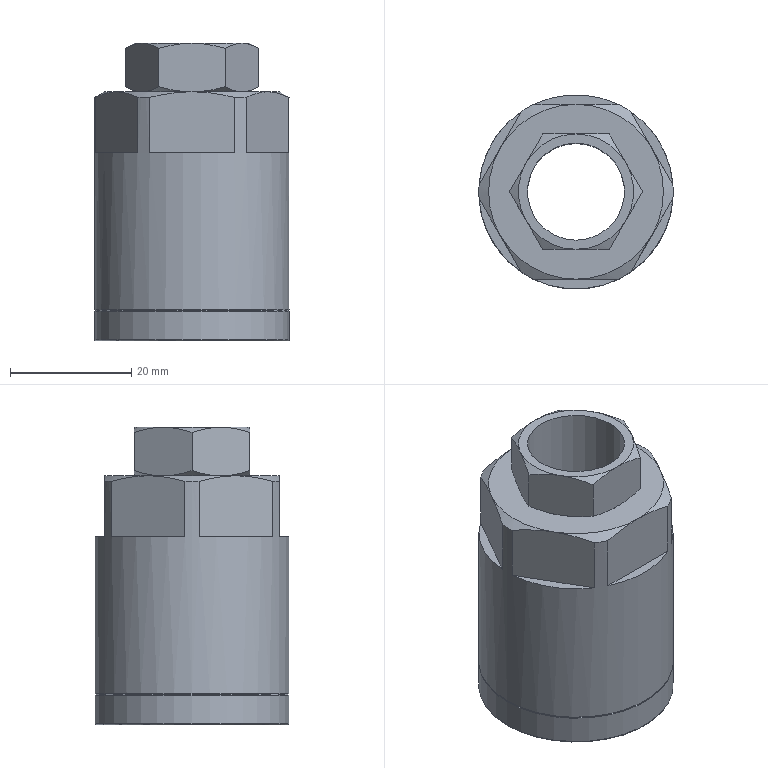Part | STEP file | 冲床-300配套压波_id654_x_t | 1 solid | 45 faces | box 32 x 32 x 49 mm | volume 24682 mm3 | plane 21 | cone 20 | cylinder 3 | torus 1 | commonest cylinder face diameters 32 x2 16 x1
STEP:
#1=CARTESIAN_POINT('',(1821.,0.,307.2));
#2=VERTEX_POINT('',#1);
#3=CARTESIAN_POINT('',(1805.,0.,307.2));
#4=DIRECTION('',(0.,0.,1.));
#5=DIRECTION('',(1.,0.,0.));
#6=AXIS2_PLACEMENT_3D('',#3,#4,#5);
#7=CIRCLE('',#6,16.);
#8=EDGE_CURVE('',#2,#2,#7,.T.);
#9=ORIENTED_EDGE('',*,*,#8,.T.);
#10=EDGE_LOOP('',(#9));
#11=FACE_BOUND('',#10,.T.);
#12=CARTESIAN_POINT('',(1789.,0.,311.9));
#13=VERTEX_POINT('',#12);
#14=CARTESIAN_POINT('',(1805.,0.,311.9));
#15=DIRECTION('',(0.,0.,-1.));
#16=DIRECTION('',(-1.,0.,0.));
#17=AXIS2_PLACEMENT_3D('',#14,#15,#16);
#18=CIRCLE('',#17,16.);
#19=EDGE_CURVE('',#13,#13,#18,.T.);
#20=ORIENTED_EDGE('',*,*,#19,.T.);
#21=EDGE_LOOP('',(#20));
#22=FACE_BOUND('',#21,.T.);
#23=CARTESIAN_POINT('',(1805.,0.,307.));
#24=DIRECTION('',(0.,0.,1.));
#25=DIRECTION('',(-1.,0.,0.));
#26=AXIS2_PLACEMENT_3D('',#23,#24,#25);
#27=CYLINDRICAL_SURFACE('',#26,16.);
#28=ADVANCED_FACE('',(#11,#22),#27,.T.);
#29=CARTESIAN_POINT('',(1813.227,4.75,348.));
#30=VERTEX_POINT('',#29);
#31=CARTESIAN_POINT('',(1805.,9.5,348.));
#32=VERTEX_POINT('',#31);
#33=CARTESIAN_POINT('',(1805.,0.,348.));
#34=DIRECTION('',(0.,0.,1.));
#35=DIRECTION('',(1.,0.,0.));
#36=AXIS2_PLACEMENT_3D('',#33,#34,#35);
#37=CIRCLE('',#36,9.5);
#38=EDGE_CURVE('',#30,#32,#37,.T.);
#39=ORIENTED_EDGE('',*,*,#38,.F.);
#40=CARTESIAN_POINT('',(1813.227,-4.75,348.));
#41=VERTEX_POINT('',#40);
#42=CARTESIAN_POINT('',(1805.,0.,348.));
#43=DIRECTION('',(0.,0.,1.));
#44=DIRECTION('',(1.,0.,0.));
#45=AXIS2_PLACEMENT_3D('',#42,#43,#44);
#46=CIRCLE('',#45,9.5);
#47=EDGE_CURVE('',#41,#30,#46,.T.);
#48=ORIENTED_EDGE('',*,*,#47,.F.);
#49=CARTESIAN_POINT('',(1805.,-9.5,348.));
#50=VERTEX_POINT('',#49);
#51=CARTESIAN_POINT('',(1805.,0.,348.));
#52=DIRECTION('',(0.,0.,1.));
#53=DIRECTION('',(1.,0.,0.));
#54=AXIS2_PLACEMENT_3D('',#51,#52,#53);
#55=CIRCLE('',#54,9.5);
#56=EDGE_CURVE('',#50,#41,#55,.T.);
#57=ORIENTED_EDGE('',*,*,#56,.F.);
#58=CARTESIAN_POINT('',(1796.773,-4.75,348.));
#59=VERTEX_POINT('',#58);
#60=CARTESIAN_POINT('',(1805.,0.,348.));
#61=DIRECTION('',(0.,0.,1.));
#62=DIRECTION('',(1.,0.,0.));
#63=AXIS2_PLACEMENT_3D('',#60,#61,#62);
#64=CIRCLE('',#63,9.5);
#65=EDGE_CURVE('',#59,#50,#64,.T.);
#66=ORIENTED_EDGE('',*,*,#65,.F.);
#67=CARTESIAN_POINT('',(1796.773,4.75,348.));
#68=VERTEX_POINT('',#67);
#69=CARTESIAN_POINT('',(1805.,0.,348.));
#70=DIRECTION('',(0.,0.,1.));
#71=DIRECTION('',(1.,0.,0.));
#72=AXIS2_PLACEMENT_3D('',#69,#70,#71);
#73=CIRCLE('',#72,9.5);
#74=EDGE_CURVE('',#68,#59,#73,.T.);
#75=ORIENTED_EDGE('',*,*,#74,.F.);
#76=CARTESIAN_POINT('',(1805.,0.,348.));
#77=DIRECTION('',(0.,0.,1.));
#78=DIRECTION('',(1.,0.,0.));
#79=AXIS2_PLACEMENT_3D('',#76,#77,#78);
#80=CIRCLE('',#79,9.5);
#81=EDGE_CURVE('',#32,#68,#80,.T.);
#82=ORIENTED_EDGE('',*,*,#81,.F.);
#83=EDGE_LOOP('',(#39,#48,#57,#66,#75,#82));
#84=FACE_BOUND('',#83,.T.);
#85=CARTESIAN_POINT('',(1805.,-14.4,348.));
#86=VERTEX_POINT('',#85);
#87=CARTESIAN_POINT('',(1817.471,-7.2,348.));
#88=VERTEX_POINT('',#87);
#89=CARTESIAN_POINT('',(1805.,0.,348.));
#90=DIRECTION('',(0.,0.,1.));
#91=DIRECTION('',(1.,0.,0.));
#92=AXIS2_PLACEMENT_3D('',#89,#90,#91);
#93=CIRCLE('',#92,14.4);
#94=EDGE_CURVE('',#86,#88,#93,.T.);
#95=ORIENTED_EDGE('',*,*,#94,.T.);
#96=CARTESIAN_POINT('',(1817.471,7.2,348.));
#97=VERTEX_POINT('',#96);
#98=CARTESIAN_POINT('',(1805.,0.,348.));
#99=DIRECTION('',(0.,0.,1.));
#100=DIRECTION('',(1.,0.,0.));
#101=AXIS2_PLACEMENT_3D('',#98,#99,#100);
#102=CIRCLE('',#101,14.4);
#103=EDGE_CURVE('',#88,#97,#102,.T.);
#104=ORIENTED_EDGE('',*,*,#103,.T.);
#105=CARTESIAN_POINT('',(1805.,14.4,348.));
#106=VERTEX_POINT('',#105);
#107=CARTESIAN_POINT('',(1805.,0.,348.));
#108=DIRECTION('',(0.,0.,1.));
#109=DIRECTION('',(1.,0.,0.));
#110=AXIS2_PLACEMENT_3D('',#107,#108,#109);
#111=CIRCLE('',#110,14.4);
#112=EDGE_CURVE('',#97,#106,#111,.T.);
#113=ORIENTED_EDGE('',*,*,#112,.T.);
#114=CARTESIAN_POINT('',(1792.529,7.2,348.));
#115=VERTEX_POINT('',#114);
#116=CARTESIAN_POINT('',(1805.,0.,348.));
#117=DIRECTION('',(0.,0.,1.));
#118=DIRECTION('',(1.,0.,0.));
#119=AXIS2_PLACEMENT_3D('',#116,#117,#118);
#120=CIRCLE('',#119,14.4);
#121=EDGE_CURVE('',#106,#115,#120,.T.);
#122=ORIENTED_EDGE('',*,*,#121,.T.);
#123=CARTESIAN_POINT('',(1792.529,-7.2,348.));
#124=VERTEX_POINT('',#123);
#125=CARTESIAN_POINT('',(1805.,0.,348.));
#126=DIRECTION('',(0.,0.,1.));
#127=DIRECTION('',(1.,0.,0.));
#128=AXIS2_PLACEMENT_3D('',#125,#126,#127);
#129=CIRCLE('',#128,14.4);
#130=EDGE_CURVE('',#115,#124,#129,.T.);
#131=ORIENTED_EDGE('',*,*,#130,.T.);
#132=CARTESIAN_POINT('',(1805.,0.,348.));
#133=DIRECTION('',(0.,0.,1.));
#134=DIRECTION('',(1.,0.,0.));
#135=AXIS2_PLACEMENT_3D('',#132,#133,#134);
#136=CIRCLE('',#135,14.4);
#137=EDGE_CURVE('',#124,#86,#136,.T.);
#138=ORIENTED_EDGE('',*,*,#137,.T.);
#139=EDGE_LOOP('',(#95,#104,#113,#122,#131,#138));
#140=FACE_BOUND('',#139,.T.);
#141=CARTESIAN_POINT('',(1805.,0.,348.));
#142=DIRECTION('',(0.,0.,1.));
#143=DIRECTION('',(-1.,0.,0.));
#144=AXIS2_PLACEMENT_3D('',#141,#142,#143);
#145=PLANE('',#144);
#146=ADVANCED_FACE('',(#84,#140),#145,.T.);
#147=CARTESIAN_POINT('',(1796.016,-13.24,338.));
#148=VERTEX_POINT('',#147);
#149=CARTESIAN_POINT('',(1789.042,-1.16,338.));
#150=VERTEX_POINT('',#149);
#151=CARTESIAN_POINT('',(1796.016,-13.24,338.));
#152=DIRECTION('',(-0.5,0.866,0.));
#153=VECTOR('',#152,1.);
#154=LINE('',#151,#153);
#155=EDGE_CURVE('',#148,#150,#154,.T.);
#156=ORIENTED_EDGE('',*,*,#155,.T.);
#157=CARTESIAN_POINT('',(1805.,0.,338.));
#158=DIRECTION('',(0.,0.,-1.));
#159=DIRECTION('',(0.5,-0.866,0.));
#160=AXIS2_PLACEMENT_3D('',#157,#158,#159);
#161=CIRCLE('',#160,16.);
#162=EDGE_CURVE('',#148,#150,#161,.T.);
#163=ORIENTED_EDGE('',*,*,#162,.F.);
#164=EDGE_LOOP('',(#156,#163));
#165=FACE_OUTER_BOUND('',#164,.T.);
#166=CARTESIAN_POINT('',(1792.529,-7.2,338.));
#167=DIRECTION('',(0.,0.,1.));
#168=DIRECTION('',(-0.5,0.866,0.));
#169=AXIS2_PLACEMENT_3D('',#166,#167,#168);
#170=PLANE('',#169);
#171=ADVANCED_FACE('',(#165),#170,.T.);
#172=CARTESIAN_POINT('',(1796.016,-13.24,347.076));
#173=VERTEX_POINT('',#172);
#174=CARTESIAN_POINT('',(1796.016,-13.24,338.));
#175=DIRECTION('',(0.,0.,-1.));
#176=VECTOR('',#175,1.);
#177=LINE('',#174,#176);
#178=EDGE_CURVE('',#173,#148,#177,.T.);
#179=ORIENTED_EDGE('',*,*,#178,.F.);
#180=CARTESIAN_POINT('',(1796.016,-13.24,347.076));
#181=CARTESIAN_POINT('',(1794.872,-11.257,347.652));
#182=CARTESIAN_POINT('',(1793.712,-9.249,348.));
#183=CARTESIAN_POINT('',(1792.529,-7.2,348.));
#184=B_SPLINE_CURVE_WITH_KNOTS('',3,(#180,#181,#182,#183),.UNSPECIFIED.,.F.,.F.,(4,4),(0.,1.),.UNSPECIFIED.);
#185=EDGE_CURVE('',#173,#124,#184,.T.);
#186=ORIENTED_EDGE('',*,*,#185,.T.);
#187=CARTESIAN_POINT('',(1789.042,-1.16,347.076));
#188=VERTEX_POINT('',#187);
#189=CARTESIAN_POINT('',(1792.529,-7.2,348.));
#190=CARTESIAN_POINT('',(1791.346,-5.151,348.));
#191=CARTESIAN_POINT('',(1790.187,-3.143,347.652));
#192=CARTESIAN_POINT('',(1789.042,-1.16,347.076));
#193=B_SPLINE_CURVE_WITH_KNOTS('',3,(#189,#190,#191,#192),.UNSPECIFIED.,.F.,.F.,(4,4),(0.,1.),.UNSPECIFIED.);
#194=EDGE_CURVE('',#124,#188,#193,.T.);
#195=ORIENTED_EDGE('',*,*,#194,.T.);
#196=CARTESIAN_POINT('',(1789.042,-1.16,338.));
#197=DIRECTION('',(0.,0.,1.));
#198=VECTOR('',#197,1.);
#199=LINE('',#196,#198);
#200=EDGE_CURVE('',#150,#188,#199,.T.);
#201=ORIENTED_EDGE('',*,*,#200,.F.);
#202=ORIENTED_EDGE('',*,*,#155,.F.);
#203=EDGE_LOOP('',(#179,#186,#195,#201,#202));
#204=FACE_OUTER_BOUND('',#203,.T.);
#205=CARTESIAN_POINT('',(1796.016,-13.24,338.));
#206=DIRECTION('',(0.866,0.5,0.));
#207=DIRECTION('',(0.5,-0.866,0.));
#208=AXIS2_PLACEMENT_3D('',#205,#206,#207);
#209=PLANE('',#208);
#210=ADVANCED_FACE('',(#204),#209,.F.);
#211=CARTESIAN_POINT('',(1789.042,1.16,338.));
#212=VERTEX_POINT('',#211);
#213=CARTESIAN_POINT('',(1796.016,13.24,338.));
#214=VERTEX_POINT('',#213);
#215=CARTESIAN_POINT('',(1789.042,1.16,338.));
#216=DIRECTION('',(0.5,0.866,0.));
#217=VECTOR('',#216,1.);
#218=LINE('',#215,#217);
#219=EDGE_CURVE('',#212,#214,#218,.T.);
#220=ORIENTED_EDGE('',*,*,#219,.T.);
#221=CARTESIAN_POINT('',(1805.,0.,338.));
#222=DIRECTION('',(0.,0.,-1.));
#223=DIRECTION('',(-0.5,-0.866,0.));
#224=AXIS2_PLACEMENT_3D('',#221,#222,#223);
#225=CIRCLE('',#224,16.);
#226=EDGE_CURVE('',#212,#214,#225,.T.);
#227=ORIENTED_EDGE('',*,*,#226,.F.);
#228=EDGE_LOOP('',(#220,#227));
#229=FACE_OUTER_BOUND('',#228,.T.);
#230=CARTESIAN_POINT('',(1792.529,7.2,338.));
#231=DIRECTION('',(0.,0.,1.));
#232=DIRECTION('',(0.5,0.866,0.));
#233=AXIS2_PLACEMENT_3D('',#230,#231,#232);
#234=PLANE('',#233);
#235=ADVANCED_FACE('',(#229),#234,.T.);
#236=CARTESIAN_POINT('',(1789.042,1.16,347.076));
#237=VERTEX_POINT('',#236);
#238=CARTESIAN_POINT('',(1789.042,1.16,338.));
#239=DIRECTION('',(0.,0.,1.));
#240=VECTOR('',#239,1.);
#241=LINE('',#238,#240);
#242=EDGE_CURVE('',#212,#237,#241,.T.);
#243=ORIENTED_EDGE('',*,*,#242,.T.);
#244=CARTESIAN_POINT('',(1789.042,1.16,347.076));
#245=CARTESIAN_POINT('',(1790.187,3.143,347.652));
#246=CARTESIAN_POINT('',(1791.346,5.151,348.));
#247=CARTESIAN_POINT('',(1792.529,7.2,348.));
#248=B_SPLINE_CURVE_WITH_KNOTS('',3,(#244,#245,#246,#247),.UNSPECIFIED.,.F.,.F.,(4,4),(0.,1.),.UNSPECIFIED.);
#249=EDGE_CURVE('',#237,#115,#248,.T.);
#250=ORIENTED_EDGE('',*,*,#249,.T.);
#251=CARTESIAN_POINT('',(1796.016,13.24,347.076));
#252=VERTEX_POINT('',#251);
#253=CARTESIAN_POINT('',(1792.529,7.2,348.));
#254=CARTESIAN_POINT('',(1793.712,9.249,348.));
#255=CARTESIAN_POINT('',(1794.872,11.257,347.652));
#256=CARTESIAN_POINT('',(1796.016,13.24,347.076));
#257=B_SPLINE_CURVE_WITH_KNOTS('',3,(#253,#254,#255,#256),.UNSPECIFIED.,.F.,.F.,(4,4),(0.,1.),.UNSPECIFIED.);
#258=EDGE_CURVE('',#115,#252,#257,.T.);
#259=ORIENTED_EDGE('',*,*,#258,.T.);
#260=CARTESIAN_POINT('',(1796.016,13.24,338.));
#261=DIRECTION('',(0.,0.,-1.));
#262=VECTOR('',#261,1.);
#263=LINE('',#260,#262);
#264=EDGE_CURVE('',#252,#214,#263,.T.);
#265=ORIENTED_EDGE('',*,*,#264,.T.);
#266=ORIENTED_EDGE('',*,*,#219,.F.);
#267=EDGE_LOOP('',(#243,#250,#259,#265,#266));
#268=FACE_OUTER_BOUND('',#267,.T.);
#269=CARTESIAN_POINT('',(1789.042,1.16,338.));
#270=DIRECTION('',(0.866,-0.5,0.));
#271=DIRECTION('',(-0.5,-0.866,0.));
#272=AXIS2_PLACEMENT_3D('',#269,#270,#271);
#273=PLANE('',#272);
#274=ADVANCED_FACE('',(#268),#273,.F.);
#275=CARTESIAN_POINT('',(1798.026,14.4,338.));
#276=VERTEX_POINT('',#275);
#277=CARTESIAN_POINT('',(1811.974,14.4,338.));
#278=VERTEX_POINT('',#277);
#279=CARTESIAN_POINT('',(1798.026,14.4,338.));
#280=DIRECTION('',(1.,0.,0.));
#281=VECTOR('',#280,1.);
#282=LINE('',#279,#281);
#283=EDGE_CURVE('',#276,#278,#282,.T.);
#284=ORIENTED_EDGE('',*,*,#283,.T.);
#285=CARTESIAN_POINT('',(1805.,0.,338.));
#286=DIRECTION('',(0.,0.,-1.));
#287=DIRECTION('',(-1.,0.,0.));
#288=AXIS2_PLACEMENT_3D('',#285,#286,#287);
#289=CIRCLE('',#288,16.);
#290=EDGE_CURVE('',#276,#278,#289,.T.);
#291=ORIENTED_EDGE('',*,*,#290,.F.);
#292=EDGE_LOOP('',(#284,#291));
#293=FACE_OUTER_BOUND('',#292,.T.);
#294=CARTESIAN_POINT('',(1805.,14.4,338.));
#295=DIRECTION('',(0.,0.,1.));
#296=DIRECTION('',(1.,0.,0.));
#297=AXIS2_PLACEMENT_3D('',#294,#295,#296);
#298=PLANE('',#297);
#299=ADVANCED_FACE('',(#293),#298,.T.);
#300=CARTESIAN_POINT('',(1798.026,14.4,347.076));
#301=VERTEX_POINT('',#300);
#302=CARTESIAN_POINT('',(1798.026,14.4,338.));
#303=DIRECTION('',(0.,0.,1.));
#304=VECTOR('',#303,1.);
#305=LINE('',#302,#304);
#306=EDGE_CURVE('',#276,#301,#305,.T.);
#307=ORIENTED_EDGE('',*,*,#306,.T.);
#308=CARTESIAN_POINT('',(1798.026,14.4,347.076));
#309=CARTESIAN_POINT('',(1800.315,14.4,347.652));
#310=CARTESIAN_POINT('',(1802.634,14.4,348.));
#311=CARTESIAN_POINT('',(1805.,14.4,348.));
#312=B_SPLINE_CURVE_WITH_KNOTS('',3,(#308,#309,#310,#311),.UNSPECIFIED.,.F.,.F.,(4,4),(0.,1.),.UNSPECIFIED.);
#313=EDGE_CURVE('',#301,#106,#312,.T.);
#314=ORIENTED_EDGE('',*,*,#313,.T.);
#315=CARTESIAN_POINT('',(1811.974,14.4,347.076));
#316=VERTEX_POINT('',#315);
#317=CARTESIAN_POINT('',(1805.,14.4,348.));
#318=CARTESIAN_POINT('',(1807.366,14.4,348.));
#319=CARTESIAN_POINT('',(1809.685,14.4,347.652));
#320=CARTESIAN_POINT('',(1811.974,14.4,347.076));
#321=B_SPLINE_CURVE_WITH_KNOTS('',3,(#317,#318,#319,#320),.UNSPECIFIED.,.F.,.F.,(4,4),(0.,1.),.UNSPECIFIED.);
#322=EDGE_CURVE('',#106,#316,#321,.T.);
#323=ORIENTED_EDGE('',*,*,#322,.T.);
#324=CARTESIAN_POINT('',(1811.974,14.4,338.));
#325=DIRECTION('',(0.,0.,-1.));
#326=VECTOR('',#325,1.);
#327=LINE('',#324,#326);
#328=EDGE_CURVE('',#316,#278,#327,.T.);
#329=ORIENTED_EDGE('',*,*,#328,.T.);
#330=ORIENTED_EDGE('',*,*,#283,.F.);
#331=EDGE_LOOP('',(#307,#314,#323,#329,#330));
#332=FACE_OUTER_BOUND('',#331,.T.);
#333=CARTESIAN_POINT('',(1798.026,14.4,338.));
#334=DIRECTION('',(0.,-1.,0.));
#335=DIRECTION('',(-1.,0.,0.));
#336=AXIS2_PLACEMENT_3D('',#333,#334,#335);
#337=PLANE('',#336);
#338=ADVANCED_FACE('',(#332),#337,.F.);
#339=CARTESIAN_POINT('',(1813.984,13.24,338.));
#340=VERTEX_POINT('',#339);
#341=CARTESIAN_POINT('',(1820.958,1.16,338.));
#342=VERTEX_POINT('',#341);
#343=CARTESIAN_POINT('',(1813.984,13.24,338.));
#344=DIRECTION('',(0.5,-0.866,0.));
#345=VECTOR('',#344,1.);
#346=LINE('',#343,#345);
#347=EDGE_CURVE('',#340,#342,#346,.T.);
#348=ORIENTED_EDGE('',*,*,#347,.T.);
#349=CARTESIAN_POINT('',(1805.,0.,338.));
#350=DIRECTION('',(0.,0.,-1.));
#351=DIRECTION('',(-0.5,0.866,0.));
#352=AXIS2_PLACEMENT_3D('',#349,#350,#351);
#353=CIRCLE('',#352,16.);
#354=EDGE_CURVE('',#340,#342,#353,.T.);
#355=ORIENTED_EDGE('',*,*,#354,.F.);
#356=EDGE_LOOP('',(#348,#355));
#357=FACE_OUTER_BOUND('',#356,.T.);
#358=CARTESIAN_POINT('',(1817.471,7.2,338.));
#359=DIRECTION('',(0.,0.,1.));
#360=DIRECTION('',(0.5,-0.866,0.));
#361=AXIS2_PLACEMENT_3D('',#358,#359,#360);
#362=PLANE('',#361);
#363=ADVANCED_FACE('',(#357),#362,.T.);
#364=CARTESIAN_POINT('',(1813.984,13.24,347.076));
#365=VERTEX_POINT('',#364);
#366=CARTESIAN_POINT('',(1813.984,13.24,338.));
#367=DIRECTION('',(0.,0.,1.));
#368=VECTOR('',#367,1.);
#369=LINE('',#366,#368);
#370=EDGE_CURVE('',#340,#365,#369,.T.);
#371=ORIENTED_EDGE('',*,*,#370,.T.);
#372=CARTESIAN_POINT('',(1813.984,13.24,347.076));
#373=CARTESIAN_POINT('',(1815.128,11.257,347.652));
#374=CARTESIAN_POINT('',(1816.288,9.249,348.));
#375=CARTESIAN_POINT('',(1817.471,7.2,348.));
#376=B_SPLINE_CURVE_WITH_KNOTS('',3,(#372,#373,#374,#375),.UNSPECIFIED.,.F.,.F.,(4,4),(0.,1.),.UNSPECIFIED.);
#377=EDGE_CURVE('',#365,#97,#376,.T.);
#378=ORIENTED_EDGE('',*,*,#377,.T.);
#379=CARTESIAN_POINT('',(1820.958,1.16,347.076));
#380=VERTEX_POINT('',#379);
#381=CARTESIAN_POINT('',(1817.471,7.2,348.));
#382=CARTESIAN_POINT('',(1818.654,5.151,348.));
#383=CARTESIAN_POINT('',(1819.813,3.143,347.652));
#384=CARTESIAN_POINT('',(1820.958,1.16,347.076));
#385=B_SPLINE_CURVE_WITH_KNOTS('',3,(#381,#382,#383,#384),.UNSPECIFIED.,.F.,.F.,(4,4),(0.,1.),.UNSPECIFIED.);
#386=EDGE_CURVE('',#97,#380,#385,.T.);
#387=ORIENTED_EDGE('',*,*,#386,.T.);
#388=CARTESIAN_POINT('',(1820.958,1.16,338.));
#389=DIRECTION('',(0.,0.,-1.));
#390=VECTOR('',#389,1.);
#391=LINE('',#388,#390);
#392=EDGE_CURVE('',#380,#342,#391,.T.);
#393=ORIENTED_EDGE('',*,*,#392,.T.);
#394=ORIENTED_EDGE('',*,*,#347,.F.);
#395=EDGE_LOOP('',(#371,#378,#387,#393,#394));
#396=FACE_OUTER_BOUND('',#395,.T.);
#397=CARTESIAN_POINT('',(1813.984,13.24,338.));
#398=DIRECTION('',(-0.866,-0.5,0.));
#399=DIRECTION('',(-0.5,0.866,0.));
#400=AXIS2_PLACEMENT_3D('',#397,#398,#399);
#401=PLANE('',#400);
#402=ADVANCED_FACE('',(#396),#401,.F.);
#403=CARTESIAN_POINT('',(1820.958,-1.16,338.));
#404=VERTEX_POINT('',#403);
#405=CARTESIAN_POINT('',(1813.984,-13.24,338.));
#406=VERTEX_POINT('',#405);
#407=CARTESIAN_POINT('',(1820.958,-1.16,338.));
#408=DIRECTION('',(-0.5,-0.866,0.));
#409=VECTOR('',#408,1.);
#410=LINE('',#407,#409);
#411=EDGE_CURVE('',#404,#406,#410,.T.);
#412=ORIENTED_EDGE('',*,*,#411,.T.);
#413=CARTESIAN_POINT('',(1805.,0.,338.));
#414=DIRECTION('',(0.,0.,-1.));
#415=DIRECTION('',(0.5,0.866,0.));
#416=AXIS2_PLACEMENT_3D('',#413,#414,#415);
#417=CIRCLE('',#416,16.);
#418=EDGE_CURVE('',#404,#406,#417,.T.);
#419=ORIENTED_EDGE('',*,*,#418,.F.);
#420=EDGE_LOOP('',(#412,#419));
#421=FACE_OUTER_BOUND('',#420,.T.);
#422=CARTESIAN_POINT('',(1817.471,-7.2,338.));
#423=DIRECTION('',(0.,0.,1.));
#424=DIRECTION('',(-0.5,-0.866,0.));
#425=AXIS2_PLACEMENT_3D('',#422,#423,#424);
#426=PLANE('',#425);
#427=ADVANCED_FACE('',(#421),#426,.T.);
#428=CARTESIAN_POINT('',(1820.958,-1.16,347.076));
#429=VERTEX_POINT('',#428);
#430=CARTESIAN_POINT('',(1820.958,-1.16,338.));
#431=DIRECTION('',(0.,0.,-1.));
#432=VECTOR('',#431,1.);
#433=LINE('',#430,#432);
#434=EDGE_CURVE('',#429,#404,#433,.T.);
#435=ORIENTED_EDGE('',*,*,#434,.F.);
#436=CARTESIAN_POINT('',(1820.958,-1.16,347.076));
#437=CARTESIAN_POINT('',(1819.813,-3.143,347.652));
#438=CARTESIAN_POINT('',(1818.654,-5.151,348.));
#439=CARTESIAN_POINT('',(1817.471,-7.2,348.));
#440=B_SPLINE_CURVE_WITH_KNOTS('',3,(#436,#437,#438,#439),.UNSPECIFIED.,.F.,.F.,(4,4),(0.,1.),.UNSPECIFIED.);
#441=EDGE_CURVE('',#429,#88,#440,.T.);
#442=ORIENTED_EDGE('',*,*,#441,.T.);
#443=CARTESIAN_POINT('',(1813.984,-13.24,347.076));
#444=VERTEX_POINT('',#443);
#445=CARTESIAN_POINT('',(1817.471,-7.2,348.));
#446=CARTESIAN_POINT('',(1816.288,-9.249,348.));
#447=CARTESIAN_POINT('',(1815.128,-11.257,347.652));
#448=CARTESIAN_POINT('',(1813.984,-13.24,347.076));
#449=B_SPLINE_CURVE_WITH_KNOTS('',3,(#445,#446,#447,#448),.UNSPECIFIED.,.F.,.F.,(4,4),(0.,1.),.UNSPECIFIED.);
#450=EDGE_CURVE('',#88,#444,#449,.T.);
#451=ORIENTED_EDGE('',*,*,#450,.T.);
#452=CARTESIAN_POINT('',(1813.984,-13.24,338.));
#453=DIRECTION('',(0.,0.,1.));
#454=VECTOR('',#453,1.);
#455=LINE('',#452,#454);
#456=EDGE_CURVE('',#406,#444,#455,.T.);
#457=ORIENTED_EDGE('',*,*,#456,.F.);
#458=ORIENTED_EDGE('',*,*,#411,.F.);
#459=EDGE_LOOP('',(#435,#442,#451,#457,#458));
#460=FACE_OUTER_BOUND('',#459,.T.);
#461=CARTESIAN_POINT('',(1820.958,-1.16,338.));
#462=DIRECTION('',(-0.866,0.5,0.));
#463=DIRECTION('',(0.5,0.866,0.));
#464=AXIS2_PLACEMENT_3D('',#461,#462,#463);
#465=PLANE('',#464);
#466=ADVANCED_FACE('',(#460),#465,.F.);
#467=CARTESIAN_POINT('',(1805.,8.,307.));
#468=VERTEX_POINT('',#467);
#469=CARTESIAN_POINT('',(1805.,0.,307.));
#470=DIRECTION('',(0.,0.,1.));
#471=DIRECTION('',(0.,1.,0.));
#472=AXIS2_PLACEMENT_3D('',#469,#470,#471);
#473=CIRCLE('',#472,8.);
#474=EDGE_CURVE('',#468,#468,#473,.T.);
#475=ORIENTED_EDGE('',*,*,#474,.F.);
#476=EDGE_LOOP('',(#475));
#477=FACE_BOUND('',#476,.T.);
#478=CARTESIAN_POINT('',(1805.,-8.,356.));
#479=VERTEX_POINT('',#478);
#480=CARTESIAN_POINT('',(1805.,0.,356.));
#481=DIRECTION('',(0.,0.,1.));
#482=DIRECTION('',(0.,-1.,0.));
#483=AXIS2_PLACEMENT_3D('',#480,#481,#482);
#484=CIRCLE('',#483,8.);
#485=EDGE_CURVE('',#479,#479,#484,.T.);
#486=ORIENTED_EDGE('',*,*,#485,.T.);
#487=EDGE_LOOP('',(#486));
#488=FACE_BOUND('',#487,.T.);
#489=CARTESIAN_POINT('',(1805.,0.,307.));
#490=DIRECTION('',(0.,0.,1.));
#491=DIRECTION('',(-1.,0.,0.));
#492=AXIS2_PLACEMENT_3D('',#489,#490,#491);
#493=CYLINDRICAL_SURFACE('',#492,8.);
#494=ADVANCED_FACE('',(#477,#488),#493,.F.);
#495=CARTESIAN_POINT('',(1789.,0.,312.1));
#496=VERTEX_POINT('',#495);
#497=CARTESIAN_POINT('',(1805.,0.,312.1));
#498=DIRECTION('',(0.,0.,-1.));
#499=DIRECTION('',(-1.,0.,0.));
#500=AXIS2_PLACEMENT_3D('',#497,#498,#499);
#501=CIRCLE('',#500,16.);
#502=EDGE_CURVE('',#496,#496,#501,.T.);
#503=ORIENTED_EDGE('',*,*,#502,.F.);
#504=EDGE_LOOP('',(#503));
#505=FACE_BOUND('',#504,.T.);
#506=CARTESIAN_POINT('',(1798.026,-14.4,347.076));
#507=VERTEX_POINT('',#506);
#508=CARTESIAN_POINT('',(1805.,0.,347.076));
#509=DIRECTION('',(0.,0.,1.));
#510=DIRECTION('',(-1.,0.,0.));
#511=AXIS2_PLACEMENT_3D('',#508,#509,#510);
#512=CIRCLE('',#511,16.);
#513=EDGE_CURVE('',#173,#507,#512,.T.);
#514=ORIENTED_EDGE('',*,*,#513,.F.);
#515=ORIENTED_EDGE('',*,*,#178,.T.);
#516=ORIENTED_EDGE('',*,*,#162,.T.);
#517=ORIENTED_EDGE('',*,*,#200,.T.);
#518=CARTESIAN_POINT('',(1805.,0.,347.076));
#519=DIRECTION('',(0.,0.,1.));
#520=DIRECTION('',(-1.,0.,0.));
#521=AXIS2_PLACEMENT_3D('',#518,#519,#520);
#522=CIRCLE('',#521,16.);
#523=EDGE_CURVE('',#237,#188,#522,.T.);
#524=ORIENTED_EDGE('',*,*,#523,.F.);
#525=ORIENTED_EDGE('',*,*,#242,.F.);
#526=ORIENTED_EDGE('',*,*,#226,.T.);
#527=ORIENTED_EDGE('',*,*,#264,.F.);
#528=CARTESIAN_POINT('',(1805.,0.,347.076));
#529=DIRECTION('',(0.,0.,1.));
#530=DIRECTION('',(-1.,0.,0.));
#531=AXIS2_PLACEMENT_3D('',#528,#529,#530);
#532=CIRCLE('',#531,16.);
#533=EDGE_CURVE('',#301,#252,#532,.T.);
#534=ORIENTED_EDGE('',*,*,#533,.F.);
#535=ORIENTED_EDGE('',*,*,#306,.F.);
#536=ORIENTED_EDGE('',*,*,#290,.T.);
#537=ORIENTED_EDGE('',*,*,#328,.F.);
#538=CARTESIAN_POINT('',(1805.,0.,347.076));
#539=DIRECTION('',(0.,0.,1.));
#540=DIRECTION('',(-1.,0.,0.));
#541=AXIS2_PLACEMENT_3D('',#538,#539,#540);
#542=CIRCLE('',#541,16.);
#543=EDGE_CURVE('',#365,#316,#542,.T.);
#544=ORIENTED_EDGE('',*,*,#543,.F.);
#545=ORIENTED_EDGE('',*,*,#370,.F.);
#546=ORIENTED_EDGE('',*,*,#354,.T.);
#547=ORIENTED_EDGE('',*,*,#392,.F.);
#548=CARTESIAN_POINT('',(1805.,0.,347.076));
#549=DIRECTION('',(0.,0.,1.));
#550=DIRECTION('',(-1.,0.,0.));
#551=AXIS2_PLACEMENT_3D('',#548,#549,#550);
#552=CIRCLE('',#551,16.);
#553=EDGE_CURVE('',#429,#380,#552,.T.);
#554=ORIENTED_EDGE('',*,*,#553,.F.);
#555=ORIENTED_EDGE('',*,*,#434,.T.);
#556=ORIENTED_EDGE('',*,*,#418,.T.);
#557=ORIENTED_EDGE('',*,*,#456,.T.);
#558=CARTESIAN_POINT('',(1811.974,-14.4,347.076));
#559=VERTEX_POINT('',#558);
#560=CARTESIAN_POINT('',(1805.,0.,347.076));
#561=DIRECTION('',(0.,0.,1.));
#562=DIRECTION('',(-1.,0.,0.));
#563=AXIS2_PLACEMENT_3D('',#560,#561,#562);
#564=CIRCLE('',#563,16.);
#565=EDGE_CURVE('',#559,#444,#564,.T.);
#566=ORIENTED_EDGE('',*,*,#565,.F.);
#567=CARTESIAN_POINT('',(1811.974,-14.4,338.));
#568=VERTEX_POINT('',#567);
#569=CARTESIAN_POINT('',(1811.974,-14.4,338.));
#570=DIRECTION('',(0.,0.,-1.));
#571=VECTOR('',#570,1.);
#572=LINE('',#569,#571);
#573=EDGE_CURVE('',#559,#568,#572,.T.);
#574=ORIENTED_EDGE('',*,*,#573,.T.);
#575=CARTESIAN_POINT('',(1798.026,-14.4,338.));
#576=VERTEX_POINT('',#575);
#577=CARTESIAN_POINT('',(1805.,0.,338.));
#578=DIRECTION('',(0.,0.,-1.));
#579=DIRECTION('',(1.,0.,0.));
#580=AXIS2_PLACEMENT_3D('',#577,#578,#579);
#581=CIRCLE('',#580,16.);
#582=EDGE_CURVE('',#568,#576,#581,.T.);
#583=ORIENTED_EDGE('',*,*,#582,.T.);
#584=CARTESIAN_POINT('',(1798.026,-14.4,338.));
#585=DIRECTION('',(0.,0.,1.));
#586=VECTOR('',#585,1.);
#587=LINE('',#584,#586);
#588=EDGE_CURVE('',#576,#507,#587,.T.);
#589=ORIENTED_EDGE('',*,*,#588,.T.);
#590=EDGE_LOOP('',(#514,#515,#516,#517,#524,#525,#526,#527,#534,#535,#536,#537,#544,#545,#546,#547,#554,#555,#556,#557,#566,#574,#583,#589));
#591=FACE_BOUND('',#590,.T.);
#592=CARTESIAN_POINT('',(1805.,0.,307.));
#593=DIRECTION('',(0.,0.,1.));
#594=DIRECTION('',(-1.,0.,0.));
#595=AXIS2_PLACEMENT_3D('',#592,#593,#594);
#596=CYLINDRICAL_SURFACE('',#595,16.);
#597=ADVANCED_FACE('',(#505,#591),#596,.T.);
#598=CARTESIAN_POINT('',(1820.8,0.,307.));
#599=VERTEX_POINT('',#598);
#600=CARTESIAN_POINT('',(1805.,0.,307.));
#601=DIRECTION('',(0.,0.,-1.));
#602=DIRECTION('',(1.,0.,0.));
#603=AXIS2_PLACEMENT_3D('',#600,#601,#602);
#604=CIRCLE('',#603,15.8);
#605=EDGE_CURVE('',#599,#599,#604,.T.);
#606=ORIENTED_EDGE('',*,*,#605,.T.);
#607=EDGE_LOOP('',(#606));
#608=FACE_BOUND('',#607,.T.);
#609=ORIENTED_EDGE('',*,*,#474,.T.);
#610=EDGE_LOOP('',(#609));
#611=FACE_BOUND('',#610,.T.);
#612=CARTESIAN_POINT('',(1805.,0.,307.));
#613=DIRECTION('',(0.,0.,1.));
#614=DIRECTION('',(-1.,0.,0.));
#615=AXIS2_PLACEMENT_3D('',#612,#613,#614);
#616=PLANE('',#615);
#617=ADVANCED_FACE('',(#608,#611),#616,.F.);
#618=CARTESIAN_POINT('',(1811.974,-14.4,338.));
#619=DIRECTION('',(-1.,0.,0.));
#620=VECTOR('',#619,1.);
#621=LINE('',#618,#620);
#622=EDGE_CURVE('',#568,#576,#621,.T.);
#623=ORIENTED_EDGE('',*,*,#622,.T.);
#624=ORIENTED_EDGE('',*,*,#582,.F.);
#625=EDGE_LOOP('',(#623,#624));
#626=FACE_OUTER_BOUND('',#625,.T.);
#627=CARTESIAN_POINT('',(1805.,-14.4,338.));
#628=DIRECTION('',(0.,0.,1.));
#629=DIRECTION('',(-1.,0.,0.));
#630=AXIS2_PLACEMENT_3D('',#627,#628,#629);
#631=PLANE('',#630);
#632=ADVANCED_FACE('',(#626),#631,.T.);
#633=ORIENTED_EDGE('',*,*,#573,.F.);
#634=CARTESIAN_POINT('',(1811.974,-14.4,347.076));
#635=CARTESIAN_POINT('',(1809.685,-14.4,347.652));
#636=CARTESIAN_POINT('',(1807.366,-14.4,348.));
#637=CARTESIAN_POINT('',(1805.,-14.4,348.));
#638=B_SPLINE_CURVE_WITH_KNOTS('',3,(#634,#635,#636,#637),.UNSPECIFIED.,.F.,.F.,(4,4),(0.,1.),.UNSPECIFIED.);
#639=EDGE_CURVE('',#559,#86,#638,.T.);
#640=ORIENTED_EDGE('',*,*,#639,.T.);
#641=CARTESIAN_POINT('',(1805.,-14.4,348.));
#642=CARTESIAN_POINT('',(1802.634,-14.4,348.));
#643=CARTESIAN_POINT('',(1800.315,-14.4,347.652));
#644=CARTESIAN_POINT('',(1798.026,-14.4,347.076));
#645=B_SPLINE_CURVE_WITH_KNOTS('',3,(#641,#642,#643,#644),.UNSPECIFIED.,.F.,.F.,(4,4),(0.,1.),.UNSPECIFIED.);
#646=EDGE_CURVE('',#86,#507,#645,.T.);
#647=ORIENTED_EDGE('',*,*,#646,.T.);
#648=ORIENTED_EDGE('',*,*,#588,.F.);
#649=ORIENTED_EDGE('',*,*,#622,.F.);
#650=EDGE_LOOP('',(#633,#640,#647,#648,#649));
#651=FACE_OUTER_BOUND('',#650,.T.);
#652=CARTESIAN_POINT('',(1811.974,-14.4,338.));
#653=DIRECTION('',(0.,1.,0.));
#654=DIRECTION('',(1.,0.,0.));
#655=AXIS2_PLACEMENT_3D('',#652,#653,#654);
#656=PLANE('',#655);
#657=ADVANCED_FACE('',(#651),#656,.F.);
#658=ORIENTED_EDGE('',*,*,#513,.T.);
#659=ORIENTED_EDGE('',*,*,#646,.F.);
#660=ORIENTED_EDGE('',*,*,#137,.F.);
#661=ORIENTED_EDGE('',*,*,#185,.F.);
#662=EDGE_LOOP('',(#658,#659,#660,#661));
#663=FACE_OUTER_BOUND('',#662,.T.);
#664=CARTESIAN_POINT('',(1805.,0.,345.5));
#665=DIRECTION('',(0.,0.,-1.));
#666=DIRECTION('',(1.,0.,0.));
#667=AXIS2_PLACEMENT_3D('',#664,#665,#666);
#668=CONICAL_SURFACE('',#667,18.73,60.);
#669=ADVANCED_FACE('',(#663),#668,.T.);
#670=ORIENTED_EDGE('',*,*,#94,.F.);
#671=ORIENTED_EDGE('',*,*,#639,.F.);
#672=ORIENTED_EDGE('',*,*,#565,.T.);
#673=ORIENTED_EDGE('',*,*,#450,.F.);
#674=EDGE_LOOP('',(#670,#671,#672,#673));
#675=FACE_OUTER_BOUND('',#674,.T.);
#676=CARTESIAN_POINT('',(1805.,0.,345.5));
#677=DIRECTION('',(0.,0.,-1.));
#678=DIRECTION('',(1.,0.,0.));
#679=AXIS2_PLACEMENT_3D('',#676,#677,#678);
#680=CONICAL_SURFACE('',#679,18.73,60.);
#681=ADVANCED_FACE('',(#675),#680,.T.);
#682=ORIENTED_EDGE('',*,*,#103,.F.);
#683=ORIENTED_EDGE('',*,*,#441,.F.);
#684=ORIENTED_EDGE('',*,*,#553,.T.);
#685=ORIENTED_EDGE('',*,*,#386,.F.);
#686=EDGE_LOOP('',(#682,#683,#684,#685));
#687=FACE_OUTER_BOUND('',#686,.T.);
#688=CARTESIAN_POINT('',(1805.,0.,345.5));
#689=DIRECTION('',(0.,0.,-1.));
#690=DIRECTION('',(1.,0.,0.));
#691=AXIS2_PLACEMENT_3D('',#688,#689,#690);
#692=CONICAL_SURFACE('',#691,18.73,60.);
#693=ADVANCED_FACE('',(#687),#692,.T.);
#694=ORIENTED_EDGE('',*,*,#112,.F.);
#695=ORIENTED_EDGE('',*,*,#377,.F.);
#696=ORIENTED_EDGE('',*,*,#543,.T.);
#697=ORIENTED_EDGE('',*,*,#322,.F.);
#698=EDGE_LOOP('',(#694,#695,#696,#697));
#699=FACE_OUTER_BOUND('',#698,.T.);
#700=CARTESIAN_POINT('',(1805.,0.,345.5));
#701=DIRECTION('',(0.,0.,-1.));
#702=DIRECTION('',(1.,0.,0.));
#703=AXIS2_PLACEMENT_3D('',#700,#701,#702);
#704=CONICAL_SURFACE('',#703,18.73,60.);
#705=ADVANCED_FACE('',(#699),#704,.T.);
#706=ORIENTED_EDGE('',*,*,#121,.F.);
#707=ORIENTED_EDGE('',*,*,#313,.F.);
#708=ORIENTED_EDGE('',*,*,#533,.T.);
#709=ORIENTED_EDGE('',*,*,#258,.F.);
#710=EDGE_LOOP('',(#706,#707,#708,#709));
#711=FACE_OUTER_BOUND('',#710,.T.);
#712=CARTESIAN_POINT('',(1805.,0.,345.5));
#713=DIRECTION('',(0.,0.,-1.));
#714=DIRECTION('',(1.,0.,0.));
#715=AXIS2_PLACEMENT_3D('',#712,#713,#714);
#716=CONICAL_SURFACE('',#715,18.73,60.);
#717=ADVANCED_FACE('',(#711),#716,.T.);
#718=ORIENTED_EDGE('',*,*,#523,.T.);
#719=ORIENTED_EDGE('',*,*,#194,.F.);
#720=ORIENTED_EDGE('',*,*,#130,.F.);
#721=ORIENTED_EDGE('',*,*,#249,.F.);
#722=EDGE_LOOP('',(#718,#719,#720,#721));
#723=FACE_OUTER_BOUND('',#722,.T.);
#724=CARTESIAN_POINT('',(1805.,0.,345.5));
#725=DIRECTION('',(0.,0.,-1.));
#726=DIRECTION('',(1.,0.,0.));
#727=AXIS2_PLACEMENT_3D('',#724,#725,#726);
#728=CONICAL_SURFACE('',#727,18.73,60.);
#729=ADVANCED_FACE('',(#723),#728,.T.);
#730=ORIENTED_EDGE('',*,*,#19,.F.);
#731=EDGE_LOOP('',(#730));
#732=FACE_BOUND('',#731,.T.);
#733=CARTESIAN_POINT('',(1789.173,0.,312.));
#734=VERTEX_POINT('',#733);
#735=CARTESIAN_POINT('',(1805.,0.,312.));
#736=DIRECTION('',(0.,0.,-1.));
#737=DIRECTION('',(-1.,0.,0.));
#738=AXIS2_PLACEMENT_3D('',#735,#736,#737);
#739=CIRCLE('',#738,15.827);
#740=EDGE_CURVE('',#734,#734,#739,.T.);
#741=ORIENTED_EDGE('',*,*,#740,.T.);
#742=EDGE_LOOP('',(#741));
#743=FACE_BOUND('',#742,.T.);
#744=CARTESIAN_POINT('',(1805.,0.,312.));
#745=DIRECTION('',(0.,0.,-1.));
#746=DIRECTION('',(1.,0.,0.));
#747=AXIS2_PLACEMENT_3D('',#744,#745,#746);
#748=CONICAL_SURFACE('',#747,15.827,60.);
#749=ADVANCED_FACE('',(#732,#743),#748,.T.);
#750=ORIENTED_EDGE('',*,*,#740,.F.);
#751=EDGE_LOOP('',(#750));
#752=FACE_BOUND('',#751,.T.);
#753=ORIENTED_EDGE('',*,*,#502,.T.);
#754=EDGE_LOOP('',(#753));
#755=FACE_BOUND('',#754,.T.);
#756=CARTESIAN_POINT('',(1805.,0.,312.1));
#757=DIRECTION('',(0.,0.,1.));
#758=DIRECTION('',(-1.,0.,0.));
#759=AXIS2_PLACEMENT_3D('',#756,#757,#758);
#760=CONICAL_SURFACE('',#759,16.,60.);
#761=ADVANCED_FACE('',(#752,#755),#760,.T.);
#762=ORIENTED_EDGE('',*,*,#605,.F.);
#763=EDGE_LOOP('',(#762));
#764=FACE_BOUND('',#763,.T.);
#765=ORIENTED_EDGE('',*,*,#8,.F.);
#766=EDGE_LOOP('',(#765));
#767=FACE_BOUND('',#766,.T.);
#768=CARTESIAN_POINT('',(1805.,0.,307.2));
#769=DIRECTION('',(0.,0.,1.));
#770=DIRECTION('',(-1.,0.,0.));
#771=AXIS2_PLACEMENT_3D('',#768,#769,#770);
#772=TOROIDAL_SURFACE('',#771,15.8,0.2);
#773=ADVANCED_FACE('',(#764,#767),#772,.T.);
#774=CARTESIAN_POINT('',(1799.515,-9.5,348.849));
#775=VERTEX_POINT('',#774);
#776=CARTESIAN_POINT('',(1799.515,-9.5,355.151));
#777=VERTEX_POINT('',#776);
#778=CARTESIAN_POINT('',(1799.515,-9.5,348.));
#779=DIRECTION('',(0.,0.,1.));
#780=VECTOR('',#779,1.);
#781=LINE('',#778,#780);
#782=EDGE_CURVE('',#775,#777,#781,.T.);
#783=ORIENTED_EDGE('',*,*,#782,.F.);
#784=CARTESIAN_POINT('',(1799.515,-9.5,348.849));
#785=CARTESIAN_POINT('',(1801.307,-9.5,348.331));
#786=CARTESIAN_POINT('',(1803.128,-9.5,348.));
#787=CARTESIAN_POINT('',(1805.,-9.5,348.));
#788=B_SPLINE_CURVE_WITH_KNOTS('',3,(#784,#785,#786,#787),.UNSPECIFIED.,.F.,.F.,(4,4),(0.,1.),.UNSPECIFIED.);
#789=EDGE_CURVE('',#775,#50,#788,.T.);
#790=ORIENTED_EDGE('',*,*,#789,.T.);
#791=CARTESIAN_POINT('',(1810.485,-9.5,348.849));
#792=VERTEX_POINT('',#791);
#793=CARTESIAN_POINT('',(1805.,-9.5,348.));
#794=CARTESIAN_POINT('',(1806.872,-9.5,348.));
#795=CARTESIAN_POINT('',(1808.693,-9.5,348.331));
#796=CARTESIAN_POINT('',(1810.485,-9.5,348.849));
#797=B_SPLINE_CURVE_WITH_KNOTS('',3,(#793,#794,#795,#796),.UNSPECIFIED.,.F.,.F.,(4,4),(0.,1.),.UNSPECIFIED.);
#798=EDGE_CURVE('',#50,#792,#797,.T.);
#799=ORIENTED_EDGE('',*,*,#798,.T.);
#800=CARTESIAN_POINT('',(1810.485,-9.5,355.151));
#801=VERTEX_POINT('',#800);
#802=CARTESIAN_POINT('',(1810.485,-9.5,348.));
#803=DIRECTION('',(0.,0.,1.));
#804=VECTOR('',#803,1.);
#805=LINE('',#802,#804);
#806=EDGE_CURVE('',#792,#801,#805,.T.);
#807=ORIENTED_EDGE('',*,*,#806,.T.);
#808=CARTESIAN_POINT('',(1805.,-9.5,356.));
#809=VERTEX_POINT('',#808);
#810=CARTESIAN_POINT('',(1805.,-9.5,356.));
#811=CARTESIAN_POINT('',(1806.872,-9.5,356.));
#812=CARTESIAN_POINT('',(1808.693,-9.5,355.669));
#813=CARTESIAN_POINT('',(1810.485,-9.5,355.151));
#814=B_SPLINE_CURVE_WITH_KNOTS('',3,(#810,#811,#812,#813),.UNSPECIFIED.,.F.,.F.,(4,4),(0.,1.),.UNSPECIFIED.);
#815=EDGE_CURVE('',#809,#801,#814,.T.);
#816=ORIENTED_EDGE('',*,*,#815,.F.);
#817=CARTESIAN_POINT('',(1799.515,-9.5,355.151));
#818=CARTESIAN_POINT('',(1801.307,-9.5,355.669));
#819=CARTESIAN_POINT('',(1803.128,-9.5,356.));
#820=CARTESIAN_POINT('',(1805.,-9.5,356.));
#821=B_SPLINE_CURVE_WITH_KNOTS('',3,(#817,#818,#819,#820),.UNSPECIFIED.,.F.,.F.,(4,4),(0.,1.),.UNSPECIFIED.);
#822=EDGE_CURVE('',#777,#809,#821,.T.);
#823=ORIENTED_EDGE('',*,*,#822,.F.);
#824=EDGE_LOOP('',(#783,#790,#799,#807,#816,#823));
#825=FACE_OUTER_BOUND('',#824,.T.);
#826=CARTESIAN_POINT('',(1799.515,-9.5,348.));
#827=DIRECTION('',(0.,-1.,0.));
#828=DIRECTION('',(-1.,0.,0.));
#829=AXIS2_PLACEMENT_3D('',#826,#827,#828);
#830=PLANE('',#829);
#831=ADVANCED_FACE('',(#825),#830,.T.);
#832=ORIENTED_EDGE('',*,*,#806,.F.);
#833=CARTESIAN_POINT('',(1810.485,-9.5,348.849));
#834=CARTESIAN_POINT('',(1811.381,-7.948,348.331));
#835=CARTESIAN_POINT('',(1812.291,-6.371,348.));
#836=CARTESIAN_POINT('',(1813.227,-4.75,348.));
#837=B_SPLINE_CURVE_WITH_KNOTS('',3,(#833,#834,#835,#836),.UNSPECIFIED.,.F.,.F.,(4,4),(0.,1.),.UNSPECIFIED.);
#838=EDGE_CURVE('',#792,#41,#837,.T.);
#839=ORIENTED_EDGE('',*,*,#838,.T.);
#840=CARTESIAN_POINT('',(1815.97,0.,348.849));
#841=VERTEX_POINT('',#840);
#842=CARTESIAN_POINT('',(1813.227,-4.75,348.));
#843=CARTESIAN_POINT('',(1814.163,-3.129,348.));
#844=CARTESIAN_POINT('',(1815.074,-1.552,348.331));
#845=CARTESIAN_POINT('',(1815.97,0.,348.849));
#846=B_SPLINE_CURVE_WITH_KNOTS('',3,(#842,#843,#844,#845),.UNSPECIFIED.,.F.,.F.,(4,4),(0.,1.),.UNSPECIFIED.);
#847=EDGE_CURVE('',#41,#841,#846,.T.);
#848=ORIENTED_EDGE('',*,*,#847,.T.);
#849=CARTESIAN_POINT('',(1815.97,0.,355.151));
#850=VERTEX_POINT('',#849);
#851=CARTESIAN_POINT('',(1815.97,0.,348.));
#852=DIRECTION('',(0.,0.,1.));
#853=VECTOR('',#852,1.);
#854=LINE('',#851,#853);
#855=EDGE_CURVE('',#841,#850,#854,.T.);
#856=ORIENTED_EDGE('',*,*,#855,.T.);
#857=CARTESIAN_POINT('',(1813.227,-4.75,356.));
#858=VERTEX_POINT('',#857);
#859=CARTESIAN_POINT('',(1813.227,-4.75,356.));
#860=CARTESIAN_POINT('',(1814.163,-3.129,356.));
#861=CARTESIAN_POINT('',(1815.074,-1.552,355.669));
#862=CARTESIAN_POINT('',(1815.97,0.,355.151));
#863=B_SPLINE_CURVE_WITH_KNOTS('',3,(#859,#860,#861,#862),.UNSPECIFIED.,.F.,.F.,(4,4),(0.,1.),.UNSPECIFIED.);
#864=EDGE_CURVE('',#858,#850,#863,.T.);
#865=ORIENTED_EDGE('',*,*,#864,.F.);
#866=CARTESIAN_POINT('',(1810.485,-9.5,355.151));
#867=CARTESIAN_POINT('',(1811.381,-7.948,355.669));
#868=CARTESIAN_POINT('',(1812.291,-6.371,356.));
#869=CARTESIAN_POINT('',(1813.227,-4.75,356.));
#870=B_SPLINE_CURVE_WITH_KNOTS('',3,(#866,#867,#868,#869),.UNSPECIFIED.,.F.,.F.,(4,4),(0.,1.),.UNSPECIFIED.);
#871=EDGE_CURVE('',#801,#858,#870,.T.);
#872=ORIENTED_EDGE('',*,*,#871,.F.);
#873=EDGE_LOOP('',(#832,#839,#848,#856,#865,#872));
#874=FACE_OUTER_BOUND('',#873,.T.);
#875=CARTESIAN_POINT('',(1810.485,-9.5,348.));
#876=DIRECTION('',(0.866,-0.5,0.));
#877=DIRECTION('',(-0.5,-0.866,0.));
#878=AXIS2_PLACEMENT_3D('',#875,#876,#877);
#879=PLANE('',#878);
#880=ADVANCED_FACE('',(#874),#879,.T.);
#881=ORIENTED_EDGE('',*,*,#855,.F.);
#882=CARTESIAN_POINT('',(1815.97,0.,348.849));
#883=CARTESIAN_POINT('',(1815.074,1.552,348.331));
#884=CARTESIAN_POINT('',(1814.163,3.129,348.));
#885=CARTESIAN_POINT('',(1813.227,4.75,348.));
#886=B_SPLINE_CURVE_WITH_KNOTS('',3,(#882,#883,#884,#885),.UNSPECIFIED.,.F.,.F.,(4,4),(0.,1.),.UNSPECIFIED.);
#887=EDGE_CURVE('',#841,#30,#886,.T.);
#888=ORIENTED_EDGE('',*,*,#887,.T.);
#889=CARTESIAN_POINT('',(1810.485,9.5,348.849));
#890=VERTEX_POINT('',#889);
#891=CARTESIAN_POINT('',(1813.227,4.75,348.));
#892=CARTESIAN_POINT('',(1812.291,6.371,348.));
#893=CARTESIAN_POINT('',(1811.381,7.948,348.331));
#894=CARTESIAN_POINT('',(1810.485,9.5,348.849));
#895=B_SPLINE_CURVE_WITH_KNOTS('',3,(#891,#892,#893,#894),.UNSPECIFIED.,.F.,.F.,(4,4),(0.,1.),.UNSPECIFIED.);
#896=EDGE_CURVE('',#30,#890,#895,.T.);
#897=ORIENTED_EDGE('',*,*,#896,.T.);
#898=CARTESIAN_POINT('',(1810.485,9.5,355.151));
#899=VERTEX_POINT('',#898);
#900=CARTESIAN_POINT('',(1810.485,9.5,348.));
#901=DIRECTION('',(0.,0.,1.));
#902=VECTOR('',#901,1.);
#903=LINE('',#900,#902);
#904=EDGE_CURVE('',#890,#899,#903,.T.);
#905=ORIENTED_EDGE('',*,*,#904,.T.);
#906=CARTESIAN_POINT('',(1813.227,4.75,356.));
#907=VERTEX_POINT('',#906);
#908=CARTESIAN_POINT('',(1813.227,4.75,356.));
#909=CARTESIAN_POINT('',(1812.291,6.371,356.));
#910=CARTESIAN_POINT('',(1811.381,7.948,355.669));
#911=CARTESIAN_POINT('',(1810.485,9.5,355.151));
#912=B_SPLINE_CURVE_WITH_KNOTS('',3,(#908,#909,#910,#911),.UNSPECIFIED.,.F.,.F.,(4,4),(0.,1.),.UNSPECIFIED.);
#913=EDGE_CURVE('',#907,#899,#912,.T.);
#914=ORIENTED_EDGE('',*,*,#913,.F.);
#915=CARTESIAN_POINT('',(1815.97,0.,355.151));
#916=CARTESIAN_POINT('',(1815.074,1.552,355.669));
#917=CARTESIAN_POINT('',(1814.163,3.129,356.));
#918=CARTESIAN_POINT('',(1813.227,4.75,356.));
#919=B_SPLINE_CURVE_WITH_KNOTS('',3,(#915,#916,#917,#918),.UNSPECIFIED.,.F.,.F.,(4,4),(0.,1.),.UNSPECIFIED.);
#920=EDGE_CURVE('',#850,#907,#919,.T.);
#921=ORIENTED_EDGE('',*,*,#920,.F.);
#922=EDGE_LOOP('',(#881,#888,#897,#905,#914,#921));
#923=FACE_OUTER_BOUND('',#922,.T.);
#924=CARTESIAN_POINT('',(1815.97,0.,348.));
#925=DIRECTION('',(0.866,0.5,0.));
#926=DIRECTION('',(0.5,-0.866,0.));
#927=AXIS2_PLACEMENT_3D('',#924,#925,#926);
#928=PLANE('',#927);
#929=ADVANCED_FACE('',(#923),#928,.T.);
#930=ORIENTED_EDGE('',*,*,#904,.F.);
#931=CARTESIAN_POINT('',(1810.485,9.5,348.849));
#932=CARTESIAN_POINT('',(1808.693,9.5,348.331));
#933=CARTESIAN_POINT('',(1806.872,9.5,348.));
#934=CARTESIAN_POINT('',(1805.,9.5,348.));
#935=B_SPLINE_CURVE_WITH_KNOTS('',3,(#931,#932,#933,#934),.UNSPECIFIED.,.F.,.F.,(4,4),(0.,1.),.UNSPECIFIED.);
#936=EDGE_CURVE('',#890,#32,#935,.T.);
#937=ORIENTED_EDGE('',*,*,#936,.T.);
#938=CARTESIAN_POINT('',(1799.515,9.5,348.849));
#939=VERTEX_POINT('',#938);
#940=CARTESIAN_POINT('',(1805.,9.5,348.));
#941=CARTESIAN_POINT('',(1803.128,9.5,348.));
#942=CARTESIAN_POINT('',(1801.307,9.5,348.331));
#943=CARTESIAN_POINT('',(1799.515,9.5,348.849));
#944=B_SPLINE_CURVE_WITH_KNOTS('',3,(#940,#941,#942,#943),.UNSPECIFIED.,.F.,.F.,(4,4),(0.,1.),.UNSPECIFIED.);
#945=EDGE_CURVE('',#32,#939,#944,.T.);
#946=ORIENTED_EDGE('',*,*,#945,.T.);
#947=CARTESIAN_POINT('',(1799.515,9.5,355.151));
#948=VERTEX_POINT('',#947);
#949=CARTESIAN_POINT('',(1799.515,9.5,348.));
#950=DIRECTION('',(0.,0.,1.));
#951=VECTOR('',#950,1.);
#952=LINE('',#949,#951);
#953=EDGE_CURVE('',#939,#948,#952,.T.);
#954=ORIENTED_EDGE('',*,*,#953,.T.);
#955=CARTESIAN_POINT('',(1805.,9.5,356.));
#956=VERTEX_POINT('',#955);
#957=CARTESIAN_POINT('',(1805.,9.5,356.));
#958=CARTESIAN_POINT('',(1803.128,9.5,356.));
#959=CARTESIAN_POINT('',(1801.307,9.5,355.669));
#960=CARTESIAN_POINT('',(1799.515,9.5,355.151));
#961=B_SPLINE_CURVE_WITH_KNOTS('',3,(#957,#958,#959,#960),.UNSPECIFIED.,.F.,.F.,(4,4),(0.,1.),.UNSPECIFIED.);
#962=EDGE_CURVE('',#956,#948,#961,.T.);
#963=ORIENTED_EDGE('',*,*,#962,.F.);
#964=CARTESIAN_POINT('',(1810.485,9.5,355.151));
#965=CARTESIAN_POINT('',(1808.693,9.5,355.669));
#966=CARTESIAN_POINT('',(1806.872,9.5,356.));
#967=CARTESIAN_POINT('',(1805.,9.5,356.));
#968=B_SPLINE_CURVE_WITH_KNOTS('',3,(#964,#965,#966,#967),.UNSPECIFIED.,.F.,.F.,(4,4),(0.,1.),.UNSPECIFIED.);
#969=EDGE_CURVE('',#899,#956,#968,.T.);
#970=ORIENTED_EDGE('',*,*,#969,.F.);
#971=EDGE_LOOP('',(#930,#937,#946,#954,#963,#970));
#972=FACE_OUTER_BOUND('',#971,.T.);
#973=CARTESIAN_POINT('',(1810.485,9.5,348.));
#974=DIRECTION('',(0.,1.,0.));
#975=DIRECTION('',(1.,0.,0.));
#976=AXIS2_PLACEMENT_3D('',#973,#974,#975);
#977=PLANE('',#976);
#978=ADVANCED_FACE('',(#972),#977,.T.);
#979=ORIENTED_EDGE('',*,*,#953,.F.);
#980=CARTESIAN_POINT('',(1799.515,9.5,348.849));
#981=CARTESIAN_POINT('',(1798.619,7.948,348.331));
#982=CARTESIAN_POINT('',(1797.709,6.371,348.));
#983=CARTESIAN_POINT('',(1796.773,4.75,348.));
#984=B_SPLINE_CURVE_WITH_KNOTS('',3,(#980,#981,#982,#983),.UNSPECIFIED.,.F.,.F.,(4,4),(0.,1.),.UNSPECIFIED.);
#985=EDGE_CURVE('',#939,#68,#984,.T.);
#986=ORIENTED_EDGE('',*,*,#985,.T.);
#987=CARTESIAN_POINT('',(1794.03,0.,348.849));
#988=VERTEX_POINT('',#987);
#989=CARTESIAN_POINT('',(1796.773,4.75,348.));
#990=CARTESIAN_POINT('',(1795.837,3.129,348.));
#991=CARTESIAN_POINT('',(1794.926,1.552,348.331));
#992=CARTESIAN_POINT('',(1794.03,0.,348.849));
#993=B_SPLINE_CURVE_WITH_KNOTS('',3,(#989,#990,#991,#992),.UNSPECIFIED.,.F.,.F.,(4,4),(0.,1.),.UNSPECIFIED.);
#994=EDGE_CURVE('',#68,#988,#993,.T.);
#995=ORIENTED_EDGE('',*,*,#994,.T.);
#996=CARTESIAN_POINT('',(1794.03,0.,355.151));
#997=VERTEX_POINT('',#996);
#998=CARTESIAN_POINT('',(1794.03,0.,348.));
#999=DIRECTION('',(0.,0.,1.));
#1000=VECTOR('',#999,1.);
#1001=LINE('',#998,#1000);
#1002=EDGE_CURVE('',#988,#997,#1001,.T.);
#1003=ORIENTED_EDGE('',*,*,#1002,.T.);
#1004=CARTESIAN_POINT('',(1796.773,4.75,356.));
#1005=VERTEX_POINT('',#1004);
#1006=CARTESIAN_POINT('',(1796.773,4.75,356.));
#1007=CARTESIAN_POINT('',(1795.837,3.129,356.));
#1008=CARTESIAN_POINT('',(1794.926,1.552,355.669));
#1009=CARTESIAN_POINT('',(1794.03,0.,355.151));
#1010=B_SPLINE_CURVE_WITH_KNOTS('',3,(#1006,#1007,#1008,#1009),.UNSPECIFIED.,.F.,.F.,(4,4),(0.,1.),.UNSPECIFIED.);
#1011=EDGE_CURVE('',#1005,#997,#1010,.T.);
#1012=ORIENTED_EDGE('',*,*,#1011,.F.);
#1013=CARTESIAN_POINT('',(1799.515,9.5,355.151));
#1014=CARTESIAN_POINT('',(1798.619,7.948,355.669));
#1015=CARTESIAN_POINT('',(1797.709,6.371,356.));
#1016=CARTESIAN_POINT('',(1796.773,4.75,356.));
#1017=B_SPLINE_CURVE_WITH_KNOTS('',3,(#1013,#1014,#1015,#1016),.UNSPECIFIED.,.F.,.F.,(4,4),(0.,1.),.UNSPECIFIED.);
#1018=EDGE_CURVE('',#948,#1005,#1017,.T.);
#1019=ORIENTED_EDGE('',*,*,#1018,.F.);
#1020=EDGE_LOOP('',(#979,#986,#995,#1003,#1012,#1019));
#1021=FACE_OUTER_BOUND('',#1020,.T.);
#1022=CARTESIAN_POINT('',(1799.515,9.5,348.));
#1023=DIRECTION('',(-0.866,0.5,0.));
#1024=DIRECTION('',(0.5,0.866,0.));
#1025=AXIS2_PLACEMENT_3D('',#1022,#1023,#1024);
#1026=PLANE('',#1025);
#1027=ADVANCED_FACE('',(#1021),#1026,.T.);
#1028=ORIENTED_EDGE('',*,*,#1002,.F.);
#1029=CARTESIAN_POINT('',(1794.03,0.,348.849));
#1030=CARTESIAN_POINT('',(1794.926,-1.552,348.331));
#1031=CARTESIAN_POINT('',(1795.837,-3.129,348.));
#1032=CARTESIAN_POINT('',(1796.773,-4.75,348.));
#1033=B_SPLINE_CURVE_WITH_KNOTS('',3,(#1029,#1030,#1031,#1032),.UNSPECIFIED.,.F.,.F.,(4,4),(0.,1.),.UNSPECIFIED.);
#1034=EDGE_CURVE('',#988,#59,#1033,.T.);
#1035=ORIENTED_EDGE('',*,*,#1034,.T.);
#1036=CARTESIAN_POINT('',(1796.773,-4.75,348.));
#1037=CARTESIAN_POINT('',(1797.709,-6.371,348.));
#1038=CARTESIAN_POINT('',(1798.619,-7.948,348.331));
#1039=CARTESIAN_POINT('',(1799.515,-9.5,348.849));
#1040=B_SPLINE_CURVE_WITH_KNOTS('',3,(#1036,#1037,#1038,#1039),.UNSPECIFIED.,.F.,.F.,(4,4),(0.,1.),.UNSPECIFIED.);
#1041=EDGE_CURVE('',#59,#775,#1040,.T.);
#1042=ORIENTED_EDGE('',*,*,#1041,.T.);
#1043=ORIENTED_EDGE('',*,*,#782,.T.);
#1044=CARTESIAN_POINT('',(1796.773,-4.75,356.));
#1045=VERTEX_POINT('',#1044);
#1046=CARTESIAN_POINT('',(1796.773,-4.75,356.));
#1047=CARTESIAN_POINT('',(1797.709,-6.371,356.));
#1048=CARTESIAN_POINT('',(1798.619,-7.948,355.669));
#1049=CARTESIAN_POINT('',(1799.515,-9.5,355.151));
#1050=B_SPLINE_CURVE_WITH_KNOTS('',3,(#1046,#1047,#1048,#1049),.UNSPECIFIED.,.F.,.F.,(4,4),(0.,1.),.UNSPECIFIED.);
#1051=EDGE_CURVE('',#1045,#777,#1050,.T.);
#1052=ORIENTED_EDGE('',*,*,#1051,.F.);
#1053=CARTESIAN_POINT('',(1794.03,0.,355.151));
#1054=CARTESIAN_POINT('',(1794.926,-1.552,355.669));
#1055=CARTESIAN_POINT('',(1795.837,-3.129,356.));
#1056=CARTESIAN_POINT('',(1796.773,-4.75,356.));
#1057=B_SPLINE_CURVE_WITH_KNOTS('',3,(#1053,#1054,#1055,#1056),.UNSPECIFIED.,.F.,.F.,(4,4),(0.,1.),.UNSPECIFIED.);
#1058=EDGE_CURVE('',#997,#1045,#1057,.T.);
#1059=ORIENTED_EDGE('',*,*,#1058,.F.);
#1060=EDGE_LOOP('',(#1028,#1035,#1042,#1043,#1052,#1059));
#1061=FACE_OUTER_BOUND('',#1060,.T.);
#1062=CARTESIAN_POINT('',(1794.03,0.,348.));
#1063=DIRECTION('',(-0.866,-0.5,0.));
#1064=DIRECTION('',(-0.5,0.866,0.));
#1065=AXIS2_PLACEMENT_3D('',#1062,#1063,#1064);
#1066=PLANE('',#1065);
#1067=ADVANCED_FACE('',(#1061),#1066,.T.);
#1068=ORIENTED_EDGE('',*,*,#485,.F.);
#1069=EDGE_LOOP('',(#1068));
#1070=FACE_BOUND('',#1069,.T.);
#1071=CARTESIAN_POINT('',(1805.,0.,356.));
#1072=DIRECTION('',(0.,0.,-1.));
#1073=DIRECTION('',(1.,0.,0.));
#1074=AXIS2_PLACEMENT_3D('',#1071,#1072,#1073);
#1075=CIRCLE('',#1074,9.5);
#1076=EDGE_CURVE('',#858,#809,#1075,.T.);
#1077=ORIENTED_EDGE('',*,*,#1076,.F.);
#1078=CARTESIAN_POINT('',(1805.,0.,356.));
#1079=DIRECTION('',(0.,0.,-1.));
#1080=DIRECTION('',(1.,0.,0.));
#1081=AXIS2_PLACEMENT_3D('',#1078,#1079,#1080);
#1082=CIRCLE('',#1081,9.5);
#1083=EDGE_CURVE('',#907,#858,#1082,.T.);
#1084=ORIENTED_EDGE('',*,*,#1083,.F.);
#1085=CARTESIAN_POINT('',(1805.,0.,356.));
#1086=DIRECTION('',(0.,0.,-1.));
#1087=DIRECTION('',(1.,0.,0.));
#1088=AXIS2_PLACEMENT_3D('',#1085,#1086,#1087);
#1089=CIRCLE('',#1088,9.5);
#1090=EDGE_CURVE('',#956,#907,#1089,.T.);
#1091=ORIENTED_EDGE('',*,*,#1090,.F.);
#1092=CARTESIAN_POINT('',(1805.,0.,356.));
#1093=DIRECTION('',(0.,0.,1.));
#1094=DIRECTION('',(1.,0.,0.));
#1095=AXIS2_PLACEMENT_3D('',#1092,#1093,#1094);
#1096=CIRCLE('',#1095,9.5);
#1097=EDGE_CURVE('',#956,#1005,#1096,.T.);
#1098=ORIENTED_EDGE('',*,*,#1097,.T.);
#1099=CARTESIAN_POINT('',(1805.,0.,356.));
#1100=DIRECTION('',(0.,0.,-1.));
#1101=DIRECTION('',(1.,0.,0.));
#1102=AXIS2_PLACEMENT_3D('',#1099,#1100,#1101);
#1103=CIRCLE('',#1102,9.5);
#1104=EDGE_CURVE('',#1045,#1005,#1103,.T.);
#1105=ORIENTED_EDGE('',*,*,#1104,.F.);
#1106=CARTESIAN_POINT('',(1805.,0.,356.));
#1107=DIRECTION('',(0.,0.,-1.));
#1108=DIRECTION('',(1.,0.,0.));
#1109=AXIS2_PLACEMENT_3D('',#1106,#1107,#1108);
#1110=CIRCLE('',#1109,9.5);
#1111=EDGE_CURVE('',#809,#1045,#1110,.T.);
#1112=ORIENTED_EDGE('',*,*,#1111,.F.);
#1113=EDGE_LOOP('',(#1077,#1084,#1091,#1098,#1105,#1112));
#1114=FACE_BOUND('',#1113,.T.);
#1115=CARTESIAN_POINT('',(1805.,0.,356.));
#1116=DIRECTION('',(0.,0.,1.));
#1117=DIRECTION('',(-1.,0.,0.));
#1118=AXIS2_PLACEMENT_3D('',#1115,#1116,#1117);
#1119=PLANE('',#1118);
#1120=ADVANCED_FACE('',(#1070,#1114),#1119,.T.);
#1121=ORIENTED_EDGE('',*,*,#864,.T.);
#1122=ORIENTED_EDGE('',*,*,#920,.T.);
#1123=ORIENTED_EDGE('',*,*,#1083,.T.);
#1124=EDGE_LOOP('',(#1121,#1122,#1123));
#1125=FACE_OUTER_BOUND('',#1124,.T.);
#1126=CARTESIAN_POINT('',(1805.,0.,353.5));
#1127=DIRECTION('',(0.,0.,-1.));
#1128=DIRECTION('',(1.,0.,0.));
#1129=AXIS2_PLACEMENT_3D('',#1126,#1127,#1128);
#1130=CONICAL_SURFACE('',#1129,13.83,60.);
#1131=ADVANCED_FACE('',(#1125),#1130,.T.);
#1132=ORIENTED_EDGE('',*,*,#913,.T.);
#1133=ORIENTED_EDGE('',*,*,#969,.T.);
#1134=ORIENTED_EDGE('',*,*,#1090,.T.);
#1135=EDGE_LOOP('',(#1132,#1133,#1134));
#1136=FACE_OUTER_BOUND('',#1135,.T.);
#1137=CARTESIAN_POINT('',(1805.,0.,353.5));
#1138=DIRECTION('',(0.,0.,-1.));
#1139=DIRECTION('',(1.,0.,0.));
#1140=AXIS2_PLACEMENT_3D('',#1137,#1138,#1139);
#1141=CONICAL_SURFACE('',#1140,13.83,60.);
#1142=ADVANCED_FACE('',(#1136),#1141,.T.);
#1143=ORIENTED_EDGE('',*,*,#962,.T.);
#1144=ORIENTED_EDGE('',*,*,#1018,.T.);
#1145=ORIENTED_EDGE('',*,*,#1097,.F.);
#1146=EDGE_LOOP('',(#1143,#1144,#1145));
#1147=FACE_OUTER_BOUND('',#1146,.T.);
#1148=CARTESIAN_POINT('',(1805.,0.,353.5));
#1149=DIRECTION('',(0.,0.,-1.));
#1150=DIRECTION('',(1.,0.,0.));
#1151=AXIS2_PLACEMENT_3D('',#1148,#1149,#1150);
#1152=CONICAL_SURFACE('',#1151,13.83,60.);
#1153=ADVANCED_FACE('',(#1147),#1152,.T.);
#1154=ORIENTED_EDGE('',*,*,#1011,.T.);
#1155=ORIENTED_EDGE('',*,*,#1058,.T.);
#1156=ORIENTED_EDGE('',*,*,#1104,.T.);
#1157=EDGE_LOOP('',(#1154,#1155,#1156));
#1158=FACE_OUTER_BOUND('',#1157,.T.);
#1159=CARTESIAN_POINT('',(1805.,0.,353.5));
#1160=DIRECTION('',(0.,0.,-1.));
#1161=DIRECTION('',(1.,0.,0.));
#1162=AXIS2_PLACEMENT_3D('',#1159,#1160,#1161);
#1163=CONICAL_SURFACE('',#1162,13.83,60.);
#1164=ADVANCED_FACE('',(#1158),#1163,.T.);
#1165=ORIENTED_EDGE('',*,*,#822,.T.);
#1166=ORIENTED_EDGE('',*,*,#1111,.T.);
#1167=ORIENTED_EDGE('',*,*,#1051,.T.);
#1168=EDGE_LOOP('',(#1165,#1166,#1167));
#1169=FACE_OUTER_BOUND('',#1168,.T.);
#1170=CARTESIAN_POINT('',(1805.,0.,353.5));
#1171=DIRECTION('',(0.,0.,-1.));
#1172=DIRECTION('',(1.,0.,0.));
#1173=AXIS2_PLACEMENT_3D('',#1170,#1171,#1172);
#1174=CONICAL_SURFACE('',#1173,13.83,60.);
#1175=ADVANCED_FACE('',(#1169),#1174,.T.);
#1176=ORIENTED_EDGE('',*,*,#815,.T.);
#1177=ORIENTED_EDGE('',*,*,#871,.T.);
#1178=ORIENTED_EDGE('',*,*,#1076,.T.);
#1179=EDGE_LOOP('',(#1176,#1177,#1178));
#1180=FACE_OUTER_BOUND('',#1179,.T.);
#1181=CARTESIAN_POINT('',(1805.,0.,353.5));
#1182=DIRECTION('',(0.,0.,-1.));
#1183=DIRECTION('',(1.,0.,0.));
#1184=AXIS2_PLACEMENT_3D('',#1181,#1182,#1183);
#1185=CONICAL_SURFACE('',#1184,13.83,60.);
#1186=ADVANCED_FACE('',(#1180),#1185,.T.);
#1187=ORIENTED_EDGE('',*,*,#47,.T.);
#1188=ORIENTED_EDGE('',*,*,#887,.F.);
#1189=ORIENTED_EDGE('',*,*,#847,.F.);
#1190=EDGE_LOOP('',(#1187,#1188,#1189));
#1191=FACE_OUTER_BOUND('',#1190,.T.);
#1192=CARTESIAN_POINT('',(1805.,0.,350.5));
#1193=DIRECTION('',(0.,0.,1.));
#1194=DIRECTION('',(-1.,0.,0.));
#1195=AXIS2_PLACEMENT_3D('',#1192,#1193,#1194);
#1196=CONICAL_SURFACE('',#1195,13.83,60.);
#1197=ADVANCED_FACE('',(#1191),#1196,.T.);
#1198=ORIENTED_EDGE('',*,*,#56,.T.);
#1199=ORIENTED_EDGE('',*,*,#838,.F.);
#1200=ORIENTED_EDGE('',*,*,#798,.F.);
#1201=EDGE_LOOP('',(#1198,#1199,#1200));
#1202=FACE_OUTER_BOUND('',#1201,.T.);
#1203=CARTESIAN_POINT('',(1805.,0.,350.5));
#1204=DIRECTION('',(0.,0.,1.));
#1205=DIRECTION('',(-1.,0.,0.));
#1206=AXIS2_PLACEMENT_3D('',#1203,#1204,#1205);
#1207=CONICAL_SURFACE('',#1206,13.83,60.);
#1208=ADVANCED_FACE('',(#1202),#1207,.T.);
#1209=ORIENTED_EDGE('',*,*,#1041,.F.);
#1210=ORIENTED_EDGE('',*,*,#65,.T.);
#1211=ORIENTED_EDGE('',*,*,#789,.F.);
#1212=EDGE_LOOP('',(#1209,#1210,#1211));
#1213=FACE_OUTER_BOUND('',#1212,.T.);
#1214=CARTESIAN_POINT('',(1805.,0.,350.5));
#1215=DIRECTION('',(0.,0.,1.));
#1216=DIRECTION('',(-1.,0.,0.));
#1217=AXIS2_PLACEMENT_3D('',#1214,#1215,#1216);
#1218=CONICAL_SURFACE('',#1217,13.83,60.);
#1219=ADVANCED_FACE('',(#1213),#1218,.T.);
#1220=ORIENTED_EDGE('',*,*,#74,.T.);
#1221=ORIENTED_EDGE('',*,*,#1034,.F.);
#1222=ORIENTED_EDGE('',*,*,#994,.F.);
#1223=EDGE_LOOP('',(#1220,#1221,#1222));
#1224=FACE_OUTER_BOUND('',#1223,.T.);
#1225=CARTESIAN_POINT('',(1805.,0.,350.5));
#1226=DIRECTION('',(0.,0.,1.));
#1227=DIRECTION('',(-1.,0.,0.));
#1228=AXIS2_PLACEMENT_3D('',#1225,#1226,#1227);
#1229=CONICAL_SURFACE('',#1228,13.83,60.);
#1230=ADVANCED_FACE('',(#1224),#1229,.T.);
#1231=ORIENTED_EDGE('',*,*,#81,.T.);
#1232=ORIENTED_EDGE('',*,*,#985,.F.);
#1233=ORIENTED_EDGE('',*,*,#945,.F.);
#1234=EDGE_LOOP('',(#1231,#1232,#1233));
#1235=FACE_OUTER_BOUND('',#1234,.T.);
#1236=CARTESIAN_POINT('',(1805.,0.,350.5));
#1237=DIRECTION('',(0.,0.,1.));
#1238=DIRECTION('',(-1.,0.,0.));
#1239=AXIS2_PLACEMENT_3D('',#1236,#1237,#1238);
#1240=CONICAL_SURFACE('',#1239,13.83,60.);
#1241=ADVANCED_FACE('',(#1235),#1240,.T.);
#1242=ORIENTED_EDGE('',*,*,#38,.T.);
#1243=ORIENTED_EDGE('',*,*,#936,.F.);
#1244=ORIENTED_EDGE('',*,*,#896,.F.);
#1245=EDGE_LOOP('',(#1242,#1243,#1244));
#1246=FACE_OUTER_BOUND('',#1245,.T.);
#1247=CARTESIAN_POINT('',(1805.,0.,350.5));
#1248=DIRECTION('',(0.,0.,1.));
#1249=DIRECTION('',(-1.,0.,0.));
#1250=AXIS2_PLACEMENT_3D('',#1247,#1248,#1249);
#1251=CONICAL_SURFACE('',#1250,13.83,60.);
#1252=ADVANCED_FACE('',(#1246),#1251,.T.);
#1253=CLOSED_SHELL('',(#28,#146,#171,#210,#235,#274,#299,#338,#363,#402,#427,#466,#494,#597,#617,#632,#657,#669,#681,#693,#705,#717,#729,#749,#761,#773,#831,#880,#929,#978,#1027,#1067,#1120,#1131,#1142,#1153,#1164,#1175,#1186,#1197,#1208,#1219,#1230,#1241,#1252));
#1254=MANIFOLD_SOLID_BREP('',#1253);
#1255=(LENGTH_UNIT()NAMED_UNIT(*)SI_UNIT(.MILLI.,.METRE.));
#1256=UNCERTAINTY_MEASURE_WITH_UNIT(LENGTH_MEASURE(0.0508),#1255,'','');
#1257=(NAMED_UNIT(*)PLANE_ANGLE_UNIT()SI_UNIT($,.RADIAN.));
#1258=PLANE_ANGLE_MEASURE_WITH_UNIT(PLANE_ANGLE_MEASURE(0.01745),#1257);
#1259=DIMENSIONAL_EXPONENTS(0.,0.,0.,0.,0.,0.,0.);
#1260=(CONVERSION_BASED_UNIT('DEGREE',#1258)NAMED_UNIT(#1259)PLANE_ANGLE_UNIT());
#1261=(NAMED_UNIT(*)SI_UNIT($,.STERADIAN.)SOLID_ANGLE_UNIT());
#1262=(GEOMETRIC_REPRESENTATION_CONTEXT(3)GLOBAL_UNCERTAINTY_ASSIGNED_CONTEXT((#1256))GLOBAL_UNIT_ASSIGNED_CONTEXT((#1255,#1260,#1261))REPRESENTATION_CONTEXT('',''));
#1263=ADVANCED_BREP_SHAPE_REPRESENTATION('',(#1254),#1262);